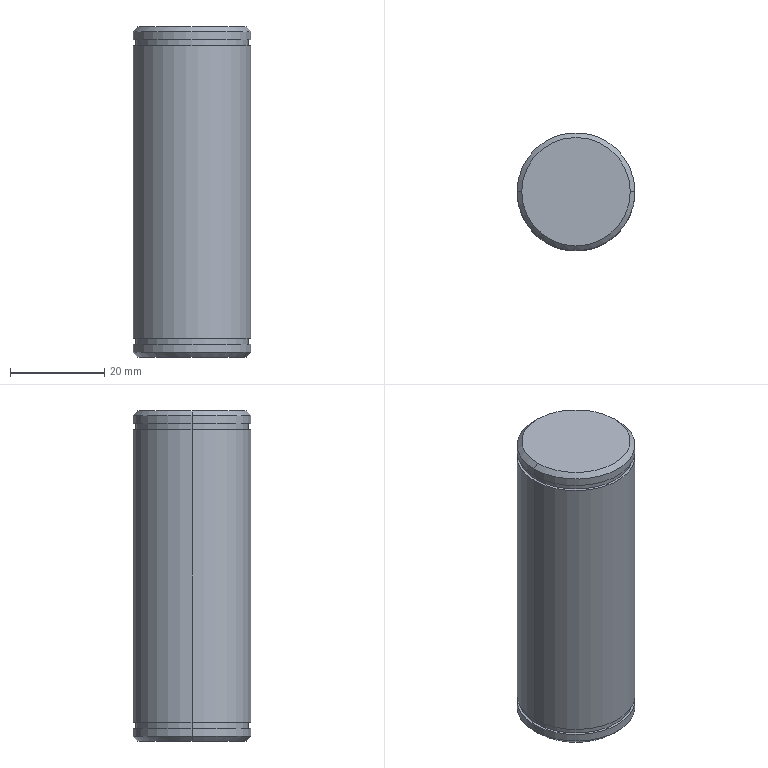Part | SolidWorks | features LibraryFeature 2, RevCut 2, Chamfer 1, Extrusion 1 | 1 solid | 20 faces | box 25 x 25 x 70 mm | volume 34175 mm3 | cylinder 10 | plane 6 | cone 4 | commonest cylinder face diameters 25 x6 23.9 x4
STEP:
#1=CARTESIAN_POINT('',(-11.5,0.,-35.));
#2=VERTEX_POINT('',#1);
#3=CARTESIAN_POINT('',(11.5,0.,-35.));
#4=VERTEX_POINT('',#3);
#5=CARTESIAN_POINT('',(0.,0.,-35.));
#6=DIRECTION('',(0.,0.,-1.));
#7=DIRECTION('',(1.,0.,0.));
#8=AXIS2_PLACEMENT_3D('',#5,#6,#7);
#9=CIRCLE('',#8,11.5);
#10=EDGE_CURVE('',#2,#4,#9,.T.);
#11=ORIENTED_EDGE('',*,*,#10,.F.);
#12=CARTESIAN_POINT('',(-12.5,0.,-34.));
#13=VERTEX_POINT('',#12);
#14=CARTESIAN_POINT('',(-12.5,0.,-34.));
#15=DIRECTION('',(-0.7071,0.,0.7071));
#16=VECTOR('',#15,1000.);
#17=LINE('',#14,#16);
#18=EDGE_CURVE('',#2,#13,#17,.T.);
#19=ORIENTED_EDGE('',*,*,#18,.T.);
#20=CARTESIAN_POINT('',(12.5,0.,-34.));
#21=VERTEX_POINT('',#20);
#22=CARTESIAN_POINT('',(0.,0.,-34.));
#23=DIRECTION('',(0.,0.,1.));
#24=DIRECTION('',(1.,0.,0.));
#25=AXIS2_PLACEMENT_3D('',#22,#23,#24);
#26=CIRCLE('',#25,12.5);
#27=EDGE_CURVE('',#21,#13,#26,.T.);
#28=ORIENTED_EDGE('',*,*,#27,.F.);
#29=CARTESIAN_POINT('',(12.5,0.,-34.));
#30=DIRECTION('',(0.7071,0.,0.7071));
#31=VECTOR('',#30,1000.);
#32=LINE('',#29,#31);
#33=EDGE_CURVE('',#4,#21,#32,.T.);
#34=ORIENTED_EDGE('',*,*,#33,.F.);
#35=EDGE_LOOP('',(#11,#19,#28,#34));
#36=FACE_OUTER_BOUND('',#35,.T.);
#37=CARTESIAN_POINT('',(0.,0.,-34.));
#38=DIRECTION('',(0.,0.,1.));
#39=DIRECTION('',(1.,0.,0.));
#40=AXIS2_PLACEMENT_3D('',#37,#38,#39);
#41=CONICAL_SURFACE('',#40,12.5,0.7854);
#42=ADVANCED_FACE('',(#36),#41,.T.);
#43=CARTESIAN_POINT('',(11.5,0.,35.));
#44=VERTEX_POINT('',#43);
#45=CARTESIAN_POINT('',(-11.5,0.,35.));
#46=VERTEX_POINT('',#45);
#47=CARTESIAN_POINT('',(0.,0.,35.));
#48=DIRECTION('',(0.,0.,1.));
#49=DIRECTION('',(1.,0.,0.));
#50=AXIS2_PLACEMENT_3D('',#47,#48,#49);
#51=CIRCLE('',#50,11.5);
#52=EDGE_CURVE('',#44,#46,#51,.T.);
#53=ORIENTED_EDGE('',*,*,#52,.F.);
#54=CARTESIAN_POINT('',(12.5,0.,34.));
#55=VERTEX_POINT('',#54);
#56=CARTESIAN_POINT('',(11.5,0.,35.));
#57=DIRECTION('',(0.7071,0.,-0.7071));
#58=VECTOR('',#57,1000.);
#59=LINE('',#56,#58);
#60=EDGE_CURVE('',#44,#55,#59,.T.);
#61=ORIENTED_EDGE('',*,*,#60,.T.);
#62=CARTESIAN_POINT('',(-12.5,0.,34.));
#63=VERTEX_POINT('',#62);
#64=CARTESIAN_POINT('',(0.,0.,34.));
#65=DIRECTION('',(0.,0.,-1.));
#66=DIRECTION('',(1.,0.,0.));
#67=AXIS2_PLACEMENT_3D('',#64,#65,#66);
#68=CIRCLE('',#67,12.5);
#69=EDGE_CURVE('',#63,#55,#68,.T.);
#70=ORIENTED_EDGE('',*,*,#69,.F.);
#71=CARTESIAN_POINT('',(-11.5,0.,35.));
#72=DIRECTION('',(-0.7071,0.,-0.7071));
#73=VECTOR('',#72,1000.);
#74=LINE('',#71,#73);
#75=EDGE_CURVE('',#46,#63,#74,.T.);
#76=ORIENTED_EDGE('',*,*,#75,.F.);
#77=EDGE_LOOP('',(#53,#61,#70,#76));
#78=FACE_OUTER_BOUND('',#77,.T.);
#79=CARTESIAN_POINT('',(0.,0.,35.));
#80=DIRECTION('',(0.,0.,-1.));
#81=DIRECTION('',(-1.,0.,0.));
#82=AXIS2_PLACEMENT_3D('',#79,#80,#81);
#83=CONICAL_SURFACE('',#82,11.5,0.7854);
#84=ADVANCED_FACE('',(#78),#83,.T.);
#85=ORIENTED_EDGE('',*,*,#69,.T.);
#86=CARTESIAN_POINT('',(12.5,0.,32.3));
#87=VERTEX_POINT('',#86);
#88=CARTESIAN_POINT('',(12.5,0.,35.));
#89=DIRECTION('',(0.,0.,-1.));
#90=VECTOR('',#89,1000.);
#91=LINE('',#88,#90);
#92=EDGE_CURVE('',#55,#87,#91,.T.);
#93=ORIENTED_EDGE('',*,*,#92,.T.);
#94=CARTESIAN_POINT('',(-12.5,0.,32.3));
#95=VERTEX_POINT('',#94);
#96=CARTESIAN_POINT('',(0.,0.,32.3));
#97=DIRECTION('',(0.,0.,1.));
#98=DIRECTION('',(1.,0.,0.));
#99=AXIS2_PLACEMENT_3D('',#96,#97,#98);
#100=CIRCLE('',#99,12.5);
#101=EDGE_CURVE('',#87,#95,#100,.T.);
#102=ORIENTED_EDGE('',*,*,#101,.T.);
#103=CARTESIAN_POINT('',(-12.5,0.,35.));
#104=DIRECTION('',(0.,0.,-1.));
#105=VECTOR('',#104,1000.);
#106=LINE('',#103,#105);
#107=EDGE_CURVE('',#63,#95,#106,.T.);
#108=ORIENTED_EDGE('',*,*,#107,.F.);
#109=EDGE_LOOP('',(#85,#93,#102,#108));
#110=FACE_OUTER_BOUND('',#109,.T.);
#111=CARTESIAN_POINT('',(0.,0.,35.));
#112=DIRECTION('',(0.,0.,-1.));
#113=DIRECTION('',(-1.,0.,0.));
#114=AXIS2_PLACEMENT_3D('',#111,#112,#113);
#115=CYLINDRICAL_SURFACE('',#114,12.5);
#116=ADVANCED_FACE('',(#110),#115,.T.);
#117=CARTESIAN_POINT('',(11.95,0.,31.));
#118=VERTEX_POINT('',#117);
#119=CARTESIAN_POINT('',(-11.95,0.,31.));
#120=VERTEX_POINT('',#119);
#121=CARTESIAN_POINT('',(0.,0.,31.));
#122=DIRECTION('',(0.,0.,1.));
#123=DIRECTION('',(1.,0.,0.));
#124=AXIS2_PLACEMENT_3D('',#121,#122,#123);
#125=CIRCLE('',#124,11.95);
#126=EDGE_CURVE('',#118,#120,#125,.T.);
#127=ORIENTED_EDGE('',*,*,#126,.T.);
#128=CARTESIAN_POINT('',(-11.95,0.,32.3));
#129=VERTEX_POINT('',#128);
#130=CARTESIAN_POINT('',(-11.95,0.,35.));
#131=DIRECTION('',(0.,0.,1.));
#132=VECTOR('',#131,1000.);
#133=LINE('',#130,#132);
#134=EDGE_CURVE('',#120,#129,#133,.T.);
#135=ORIENTED_EDGE('',*,*,#134,.T.);
#136=CARTESIAN_POINT('',(11.95,0.,32.3));
#137=VERTEX_POINT('',#136);
#138=CARTESIAN_POINT('',(0.,0.,32.3));
#139=DIRECTION('',(0.,0.,1.));
#140=DIRECTION('',(1.,0.,0.));
#141=AXIS2_PLACEMENT_3D('',#138,#139,#140);
#142=CIRCLE('',#141,11.95);
#143=EDGE_CURVE('',#137,#129,#142,.T.);
#144=ORIENTED_EDGE('',*,*,#143,.F.);
#145=CARTESIAN_POINT('',(11.95,0.,35.));
#146=DIRECTION('',(0.,0.,1.));
#147=VECTOR('',#146,1000.);
#148=LINE('',#145,#147);
#149=EDGE_CURVE('',#118,#137,#148,.T.);
#150=ORIENTED_EDGE('',*,*,#149,.F.);
#151=EDGE_LOOP('',(#127,#135,#144,#150));
#152=FACE_OUTER_BOUND('',#151,.T.);
#153=CARTESIAN_POINT('',(0.,0.,35.));
#154=DIRECTION('',(0.,0.,1.));
#155=DIRECTION('',(1.,0.,0.));
#156=AXIS2_PLACEMENT_3D('',#153,#154,#155);
#157=CYLINDRICAL_SURFACE('',#156,11.95);
#158=ADVANCED_FACE('',(#152),#157,.T.);
#159=CARTESIAN_POINT('',(12.5,0.,31.));
#160=VERTEX_POINT('',#159);
#161=CARTESIAN_POINT('',(-12.5,0.,31.));
#162=VERTEX_POINT('',#161);
#163=CARTESIAN_POINT('',(0.,0.,31.));
#164=DIRECTION('',(0.,0.,1.));
#165=DIRECTION('',(1.,0.,0.));
#166=AXIS2_PLACEMENT_3D('',#163,#164,#165);
#167=CIRCLE('',#166,12.5);
#168=EDGE_CURVE('',#160,#162,#167,.T.);
#169=ORIENTED_EDGE('',*,*,#168,.F.);
#170=CARTESIAN_POINT('',(12.5,0.,-31.));
#171=VERTEX_POINT('',#170);
#172=CARTESIAN_POINT('',(12.5,0.,35.));
#173=DIRECTION('',(0.,0.,-1.));
#174=VECTOR('',#173,1000.);
#175=LINE('',#172,#174);
#176=EDGE_CURVE('',#160,#171,#175,.T.);
#177=ORIENTED_EDGE('',*,*,#176,.T.);
#178=CARTESIAN_POINT('',(-12.5,0.,-31.));
#179=VERTEX_POINT('',#178);
#180=CARTESIAN_POINT('',(0.,0.,-31.));
#181=DIRECTION('',(0.,0.,-1.));
#182=DIRECTION('',(-1.,0.,0.));
#183=AXIS2_PLACEMENT_3D('',#180,#181,#182);
#184=CIRCLE('',#183,12.5);
#185=EDGE_CURVE('',#179,#171,#184,.T.);
#186=ORIENTED_EDGE('',*,*,#185,.F.);
#187=CARTESIAN_POINT('',(-12.5,0.,35.));
#188=DIRECTION('',(0.,0.,-1.));
#189=VECTOR('',#188,1000.);
#190=LINE('',#187,#189);
#191=EDGE_CURVE('',#162,#179,#190,.T.);
#192=ORIENTED_EDGE('',*,*,#191,.F.);
#193=EDGE_LOOP('',(#169,#177,#186,#192));
#194=FACE_OUTER_BOUND('',#193,.T.);
#195=CARTESIAN_POINT('',(0.,0.,35.));
#196=DIRECTION('',(0.,0.,-1.));
#197=DIRECTION('',(-1.,0.,0.));
#198=AXIS2_PLACEMENT_3D('',#195,#196,#197);
#199=CYLINDRICAL_SURFACE('',#198,12.5);
#200=ADVANCED_FACE('',(#194),#199,.T.);
#201=CARTESIAN_POINT('',(-11.95,0.,-31.));
#202=VERTEX_POINT('',#201);
#203=CARTESIAN_POINT('',(11.95,0.,-31.));
#204=VERTEX_POINT('',#203);
#205=CARTESIAN_POINT('',(0.,0.,-31.));
#206=DIRECTION('',(0.,0.,-1.));
#207=DIRECTION('',(-1.,0.,0.));
#208=AXIS2_PLACEMENT_3D('',#205,#206,#207);
#209=CIRCLE('',#208,11.95);
#210=EDGE_CURVE('',#202,#204,#209,.T.);
#211=ORIENTED_EDGE('',*,*,#210,.T.);
#212=CARTESIAN_POINT('',(11.95,0.,-32.3));
#213=VERTEX_POINT('',#212);
#214=CARTESIAN_POINT('',(11.95,0.,-35.));
#215=DIRECTION('',(0.,0.,-1.));
#216=VECTOR('',#215,1000.);
#217=LINE('',#214,#216);
#218=EDGE_CURVE('',#204,#213,#217,.T.);
#219=ORIENTED_EDGE('',*,*,#218,.T.);
#220=CARTESIAN_POINT('',(-11.95,0.,-32.3));
#221=VERTEX_POINT('',#220);
#222=CARTESIAN_POINT('',(0.,0.,-32.3));
#223=DIRECTION('',(0.,0.,-1.));
#224=DIRECTION('',(-1.,0.,0.));
#225=AXIS2_PLACEMENT_3D('',#222,#223,#224);
#226=CIRCLE('',#225,11.95);
#227=EDGE_CURVE('',#221,#213,#226,.T.);
#228=ORIENTED_EDGE('',*,*,#227,.F.);
#229=CARTESIAN_POINT('',(-11.95,0.,-35.));
#230=DIRECTION('',(0.,0.,-1.));
#231=VECTOR('',#230,1000.);
#232=LINE('',#229,#231);
#233=EDGE_CURVE('',#202,#221,#232,.T.);
#234=ORIENTED_EDGE('',*,*,#233,.F.);
#235=EDGE_LOOP('',(#211,#219,#228,#234));
#236=FACE_OUTER_BOUND('',#235,.T.);
#237=CARTESIAN_POINT('',(0.,0.,-35.));
#238=DIRECTION('',(0.,0.,-1.));
#239=DIRECTION('',(-1.,0.,0.));
#240=AXIS2_PLACEMENT_3D('',#237,#238,#239);
#241=CYLINDRICAL_SURFACE('',#240,11.95);
#242=ADVANCED_FACE('',(#236),#241,.T.);
#243=CARTESIAN_POINT('',(-12.5,0.,-32.3));
#244=VERTEX_POINT('',#243);
#245=CARTESIAN_POINT('',(12.5,0.,-32.3));
#246=VERTEX_POINT('',#245);
#247=CARTESIAN_POINT('',(0.,0.,-32.3));
#248=DIRECTION('',(0.,0.,-1.));
#249=DIRECTION('',(-1.,0.,0.));
#250=AXIS2_PLACEMENT_3D('',#247,#248,#249);
#251=CIRCLE('',#250,12.5);
#252=EDGE_CURVE('',#244,#246,#251,.T.);
#253=ORIENTED_EDGE('',*,*,#252,.T.);
#254=CARTESIAN_POINT('',(12.5,0.,35.));
#255=DIRECTION('',(0.,0.,-1.));
#256=VECTOR('',#255,1000.);
#257=LINE('',#254,#256);
#258=EDGE_CURVE('',#246,#21,#257,.T.);
#259=ORIENTED_EDGE('',*,*,#258,.T.);
#260=ORIENTED_EDGE('',*,*,#27,.T.);
#261=CARTESIAN_POINT('',(-12.5,0.,35.));
#262=DIRECTION('',(0.,0.,-1.));
#263=VECTOR('',#262,1000.);
#264=LINE('',#261,#263);
#265=EDGE_CURVE('',#244,#13,#264,.T.);
#266=ORIENTED_EDGE('',*,*,#265,.F.);
#267=EDGE_LOOP('',(#253,#259,#260,#266));
#268=FACE_OUTER_BOUND('',#267,.T.);
#269=CARTESIAN_POINT('',(0.,0.,35.));
#270=DIRECTION('',(0.,0.,-1.));
#271=DIRECTION('',(-1.,0.,0.));
#272=AXIS2_PLACEMENT_3D('',#269,#270,#271);
#273=CYLINDRICAL_SURFACE('',#272,12.5);
#274=ADVANCED_FACE('',(#268),#273,.T.);
#275=ORIENTED_EDGE('',*,*,#258,.F.);
#276=CARTESIAN_POINT('',(0.,0.,-32.3));
#277=DIRECTION('',(0.,0.,-1.));
#278=DIRECTION('',(-1.,0.,0.));
#279=AXIS2_PLACEMENT_3D('',#276,#277,#278);
#280=CIRCLE('',#279,12.5);
#281=EDGE_CURVE('',#246,#244,#280,.T.);
#282=ORIENTED_EDGE('',*,*,#281,.T.);
#283=ORIENTED_EDGE('',*,*,#265,.T.);
#284=CARTESIAN_POINT('',(0.,0.,-34.));
#285=DIRECTION('',(0.,0.,1.));
#286=DIRECTION('',(1.,0.,0.));
#287=AXIS2_PLACEMENT_3D('',#284,#285,#286);
#288=CIRCLE('',#287,12.5);
#289=EDGE_CURVE('',#13,#21,#288,.T.);
#290=ORIENTED_EDGE('',*,*,#289,.T.);
#291=EDGE_LOOP('',(#275,#282,#283,#290));
#292=FACE_OUTER_BOUND('',#291,.T.);
#293=CARTESIAN_POINT('',(0.,0.,35.));
#294=DIRECTION('',(0.,0.,-1.));
#295=DIRECTION('',(-1.,0.,0.));
#296=AXIS2_PLACEMENT_3D('',#293,#294,#295);
#297=CYLINDRICAL_SURFACE('',#296,12.5);
#298=ADVANCED_FACE('',(#292),#297,.T.);
#299=CARTESIAN_POINT('',(0.,0.,-35.));
#300=DIRECTION('',(0.,0.,-1.));
#301=DIRECTION('',(1.,0.,0.));
#302=AXIS2_PLACEMENT_3D('',#299,#300,#301);
#303=CIRCLE('',#302,11.5);
#304=EDGE_CURVE('',#4,#2,#303,.T.);
#305=ORIENTED_EDGE('',*,*,#304,.T.);
#306=ORIENTED_EDGE('',*,*,#10,.T.);
#307=EDGE_LOOP('',(#305,#306));
#308=FACE_OUTER_BOUND('',#307,.T.);
#309=CARTESIAN_POINT('',(0.,0.,-35.));
#310=DIRECTION('',(0.,0.,1.));
#311=DIRECTION('',(1.,0.,0.));
#312=AXIS2_PLACEMENT_3D('',#309,#310,#311);
#313=PLANE('',#312);
#314=ADVANCED_FACE('',(#308),#313,.F.);
#315=ORIENTED_EDGE('',*,*,#252,.F.);
#316=ORIENTED_EDGE('',*,*,#281,.F.);
#317=EDGE_LOOP('',(#315,#316));
#318=FACE_OUTER_BOUND('',#317,.T.);
#319=ORIENTED_EDGE('',*,*,#227,.T.);
#320=CARTESIAN_POINT('',(0.,0.,-32.3));
#321=DIRECTION('',(0.,0.,-1.));
#322=DIRECTION('',(-1.,0.,0.));
#323=AXIS2_PLACEMENT_3D('',#320,#321,#322);
#324=CIRCLE('',#323,11.95);
#325=EDGE_CURVE('',#213,#221,#324,.T.);
#326=ORIENTED_EDGE('',*,*,#325,.T.);
#327=EDGE_LOOP('',(#319,#326));
#328=FACE_BOUND('',#327,.T.);
#329=CARTESIAN_POINT('',(-12.5,0.,-32.3));
#330=DIRECTION('',(0.,0.,-1.));
#331=DIRECTION('',(-1.,0.,0.));
#332=AXIS2_PLACEMENT_3D('',#329,#330,#331);
#333=PLANE('',#332);
#334=ADVANCED_FACE('',(#318,#328),#333,.F.);
#335=ORIENTED_EDGE('',*,*,#218,.F.);
#336=CARTESIAN_POINT('',(0.,0.,-31.));
#337=DIRECTION('',(0.,0.,-1.));
#338=DIRECTION('',(-1.,0.,0.));
#339=AXIS2_PLACEMENT_3D('',#336,#337,#338);
#340=CIRCLE('',#339,11.95);
#341=EDGE_CURVE('',#204,#202,#340,.T.);
#342=ORIENTED_EDGE('',*,*,#341,.T.);
#343=ORIENTED_EDGE('',*,*,#233,.T.);
#344=ORIENTED_EDGE('',*,*,#325,.F.);
#345=EDGE_LOOP('',(#335,#342,#343,#344));
#346=FACE_OUTER_BOUND('',#345,.T.);
#347=CARTESIAN_POINT('',(0.,0.,-35.));
#348=DIRECTION('',(0.,0.,-1.));
#349=DIRECTION('',(-1.,0.,0.));
#350=AXIS2_PLACEMENT_3D('',#347,#348,#349);
#351=CYLINDRICAL_SURFACE('',#350,11.95);
#352=ADVANCED_FACE('',(#346),#351,.T.);
#353=ORIENTED_EDGE('',*,*,#210,.F.);
#354=ORIENTED_EDGE('',*,*,#341,.F.);
#355=EDGE_LOOP('',(#353,#354));
#356=FACE_BOUND('',#355,.T.);
#357=ORIENTED_EDGE('',*,*,#185,.T.);
#358=CARTESIAN_POINT('',(0.,0.,-31.));
#359=DIRECTION('',(0.,0.,-1.));
#360=DIRECTION('',(-1.,0.,0.));
#361=AXIS2_PLACEMENT_3D('',#358,#359,#360);
#362=CIRCLE('',#361,12.5);
#363=EDGE_CURVE('',#171,#179,#362,.T.);
#364=ORIENTED_EDGE('',*,*,#363,.T.);
#365=EDGE_LOOP('',(#357,#364));
#366=FACE_OUTER_BOUND('',#365,.T.);
#367=CARTESIAN_POINT('',(-12.5,0.,-31.));
#368=DIRECTION('',(0.,0.,1.));
#369=DIRECTION('',(1.,0.,0.));
#370=AXIS2_PLACEMENT_3D('',#367,#368,#369);
#371=PLANE('',#370);
#372=ADVANCED_FACE('',(#356,#366),#371,.F.);
#373=ORIENTED_EDGE('',*,*,#176,.F.);
#374=CARTESIAN_POINT('',(0.,0.,31.));
#375=DIRECTION('',(0.,0.,1.));
#376=DIRECTION('',(1.,0.,0.));
#377=AXIS2_PLACEMENT_3D('',#374,#375,#376);
#378=CIRCLE('',#377,12.5);
#379=EDGE_CURVE('',#162,#160,#378,.T.);
#380=ORIENTED_EDGE('',*,*,#379,.F.);
#381=ORIENTED_EDGE('',*,*,#191,.T.);
#382=ORIENTED_EDGE('',*,*,#363,.F.);
#383=EDGE_LOOP('',(#373,#380,#381,#382));
#384=FACE_OUTER_BOUND('',#383,.T.);
#385=CARTESIAN_POINT('',(0.,0.,35.));
#386=DIRECTION('',(0.,0.,-1.));
#387=DIRECTION('',(-1.,0.,0.));
#388=AXIS2_PLACEMENT_3D('',#385,#386,#387);
#389=CYLINDRICAL_SURFACE('',#388,12.5);
#390=ADVANCED_FACE('',(#384),#389,.T.);
#391=CARTESIAN_POINT('',(0.,0.,32.3));
#392=DIRECTION('',(0.,0.,1.));
#393=DIRECTION('',(1.,0.,0.));
#394=AXIS2_PLACEMENT_3D('',#391,#392,#393);
#395=CIRCLE('',#394,12.5);
#396=EDGE_CURVE('',#95,#87,#395,.T.);
#397=ORIENTED_EDGE('',*,*,#396,.F.);
#398=ORIENTED_EDGE('',*,*,#101,.F.);
#399=EDGE_LOOP('',(#397,#398));
#400=FACE_OUTER_BOUND('',#399,.T.);
#401=ORIENTED_EDGE('',*,*,#143,.T.);
#402=CARTESIAN_POINT('',(0.,0.,32.3));
#403=DIRECTION('',(0.,0.,1.));
#404=DIRECTION('',(1.,0.,0.));
#405=AXIS2_PLACEMENT_3D('',#402,#403,#404);
#406=CIRCLE('',#405,11.95);
#407=EDGE_CURVE('',#129,#137,#406,.T.);
#408=ORIENTED_EDGE('',*,*,#407,.T.);
#409=EDGE_LOOP('',(#401,#408));
#410=FACE_BOUND('',#409,.T.);
#411=CARTESIAN_POINT('',(12.5,0.,32.3));
#412=DIRECTION('',(0.,0.,1.));
#413=DIRECTION('',(1.,0.,0.));
#414=AXIS2_PLACEMENT_3D('',#411,#412,#413);
#415=PLANE('',#414);
#416=ADVANCED_FACE('',(#400,#410),#415,.F.);
#417=ORIENTED_EDGE('',*,*,#134,.F.);
#418=CARTESIAN_POINT('',(0.,0.,31.));
#419=DIRECTION('',(0.,0.,1.));
#420=DIRECTION('',(1.,0.,0.));
#421=AXIS2_PLACEMENT_3D('',#418,#419,#420);
#422=CIRCLE('',#421,11.95);
#423=EDGE_CURVE('',#120,#118,#422,.T.);
#424=ORIENTED_EDGE('',*,*,#423,.T.);
#425=ORIENTED_EDGE('',*,*,#149,.T.);
#426=ORIENTED_EDGE('',*,*,#407,.F.);
#427=EDGE_LOOP('',(#417,#424,#425,#426));
#428=FACE_OUTER_BOUND('',#427,.T.);
#429=CARTESIAN_POINT('',(0.,0.,35.));
#430=DIRECTION('',(0.,0.,1.));
#431=DIRECTION('',(1.,0.,0.));
#432=AXIS2_PLACEMENT_3D('',#429,#430,#431);
#433=CYLINDRICAL_SURFACE('',#432,11.95);
#434=ADVANCED_FACE('',(#428),#433,.T.);
#435=ORIENTED_EDGE('',*,*,#126,.F.);
#436=ORIENTED_EDGE('',*,*,#423,.F.);
#437=EDGE_LOOP('',(#435,#436));
#438=FACE_BOUND('',#437,.T.);
#439=ORIENTED_EDGE('',*,*,#379,.T.);
#440=ORIENTED_EDGE('',*,*,#168,.T.);
#441=EDGE_LOOP('',(#439,#440));
#442=FACE_OUTER_BOUND('',#441,.T.);
#443=CARTESIAN_POINT('',(12.5,0.,31.));
#444=DIRECTION('',(0.,0.,-1.));
#445=DIRECTION('',(-1.,0.,0.));
#446=AXIS2_PLACEMENT_3D('',#443,#444,#445);
#447=PLANE('',#446);
#448=ADVANCED_FACE('',(#438,#442),#447,.F.);
#449=CARTESIAN_POINT('',(0.,0.,35.));
#450=DIRECTION('',(0.,0.,1.));
#451=DIRECTION('',(1.,0.,0.));
#452=AXIS2_PLACEMENT_3D('',#449,#450,#451);
#453=CIRCLE('',#452,11.5);
#454=EDGE_CURVE('',#46,#44,#453,.T.);
#455=ORIENTED_EDGE('',*,*,#454,.T.);
#456=ORIENTED_EDGE('',*,*,#52,.T.);
#457=EDGE_LOOP('',(#455,#456));
#458=FACE_OUTER_BOUND('',#457,.T.);
#459=CARTESIAN_POINT('',(0.,0.,35.));
#460=DIRECTION('',(0.,0.,1.));
#461=DIRECTION('',(1.,0.,0.));
#462=AXIS2_PLACEMENT_3D('',#459,#460,#461);
#463=PLANE('',#462);
#464=ADVANCED_FACE('',(#458),#463,.T.);
#465=ORIENTED_EDGE('',*,*,#92,.F.);
#466=CARTESIAN_POINT('',(0.,0.,34.));
#467=DIRECTION('',(0.,0.,-1.));
#468=DIRECTION('',(1.,0.,0.));
#469=AXIS2_PLACEMENT_3D('',#466,#467,#468);
#470=CIRCLE('',#469,12.5);
#471=EDGE_CURVE('',#55,#63,#470,.T.);
#472=ORIENTED_EDGE('',*,*,#471,.T.);
#473=ORIENTED_EDGE('',*,*,#107,.T.);
#474=ORIENTED_EDGE('',*,*,#396,.T.);
#475=EDGE_LOOP('',(#465,#472,#473,#474));
#476=FACE_OUTER_BOUND('',#475,.T.);
#477=CARTESIAN_POINT('',(0.,0.,35.));
#478=DIRECTION('',(0.,0.,-1.));
#479=DIRECTION('',(-1.,0.,0.));
#480=AXIS2_PLACEMENT_3D('',#477,#478,#479);
#481=CYLINDRICAL_SURFACE('',#480,12.5);
#482=ADVANCED_FACE('',(#476),#481,.T.);
#483=ORIENTED_EDGE('',*,*,#60,.F.);
#484=ORIENTED_EDGE('',*,*,#454,.F.);
#485=ORIENTED_EDGE('',*,*,#75,.T.);
#486=ORIENTED_EDGE('',*,*,#471,.F.);
#487=EDGE_LOOP('',(#483,#484,#485,#486));
#488=FACE_OUTER_BOUND('',#487,.T.);
#489=CARTESIAN_POINT('',(0.,0.,35.));
#490=DIRECTION('',(0.,0.,-1.));
#491=DIRECTION('',(-1.,0.,0.));
#492=AXIS2_PLACEMENT_3D('',#489,#490,#491);
#493=CONICAL_SURFACE('',#492,11.5,0.7854);
#494=ADVANCED_FACE('',(#488),#493,.T.);
#495=ORIENTED_EDGE('',*,*,#18,.F.);
#496=ORIENTED_EDGE('',*,*,#304,.F.);
#497=ORIENTED_EDGE('',*,*,#33,.T.);
#498=ORIENTED_EDGE('',*,*,#289,.F.);
#499=EDGE_LOOP('',(#495,#496,#497,#498));
#500=FACE_OUTER_BOUND('',#499,.T.);
#501=CARTESIAN_POINT('',(0.,0.,-34.));
#502=DIRECTION('',(0.,0.,1.));
#503=DIRECTION('',(1.,0.,0.));
#504=AXIS2_PLACEMENT_3D('',#501,#502,#503);
#505=CONICAL_SURFACE('',#504,12.5,0.7854);
#506=ADVANCED_FACE('',(#500),#505,.T.);
#507=CLOSED_SHELL('',(#42,#84,#116,#158,#200,#242,#274,#298,#314,#334,#352,#372,#390,#416,#434,#448,#464,#482,#494,#506));
#508=MANIFOLD_SOLID_BREP('',#507);
#509=CARTESIAN_POINT('',(0.,0.,0.));
#510=DIRECTION('',(0.,0.,1.));
#511=DIRECTION('',(1.,0.,0.));
#512=AXIS2_PLACEMENT_3D('',#509,#510,#511);
#513=(LENGTH_UNIT()NAMED_UNIT(*)SI_UNIT(.MILLI.,.METRE.));
#514=UNCERTAINTY_MEASURE_WITH_UNIT(LENGTH_MEASURE(0.00001),#513,'','');
#515=(NAMED_UNIT(*)PLANE_ANGLE_UNIT()SI_UNIT($,.RADIAN.));
#516=(NAMED_UNIT(*)SI_UNIT($,.STERADIAN.)SOLID_ANGLE_UNIT());
#517=(GEOMETRIC_REPRESENTATION_CONTEXT(3)GLOBAL_UNCERTAINTY_ASSIGNED_CONTEXT((#514))GLOBAL_UNIT_ASSIGNED_CONTEXT((#513,#515,#516))REPRESENTATION_CONTEXT('',''));
#518=ADVANCED_BREP_SHAPE_REPRESENTATION('',(#508,#512),#517);